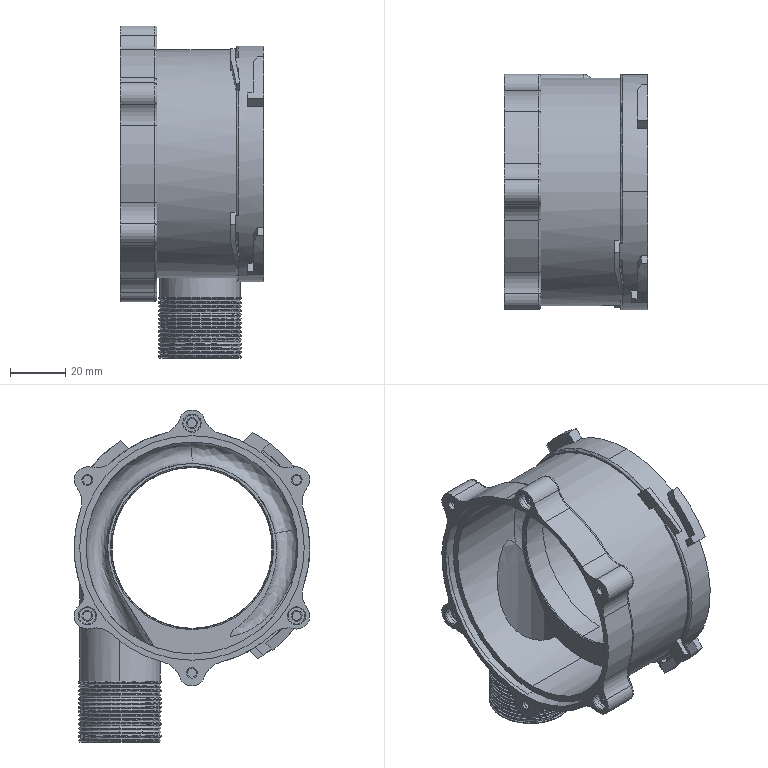Part | STEP file | 12_12-3_5 | 1 solid | 287 faces | box 51.9 x 85 x 119.75 mm | volume 69599 mm3 | torus 107 | cylinder 101 | plane 60 | spline 15 | other 2 | cone 2 | commonest cylinder face diameters 29 x32 3.3 x12 16 x11 85 x8 6 x6 9.5 x6